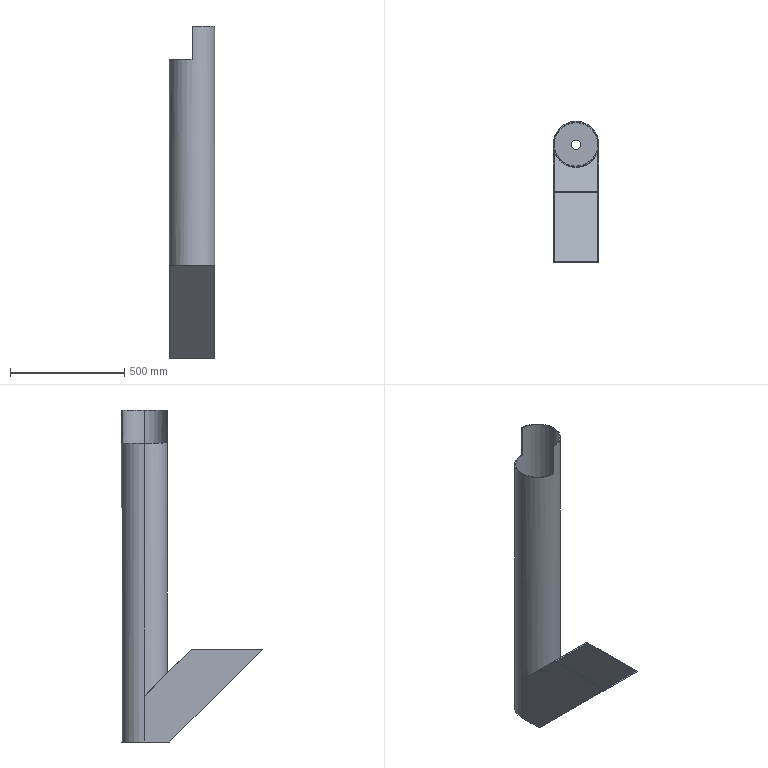Part | SolidWorks | features ICE 5, Shell 2, Extrusion 1 | 2 solids | 26 faces | box 200 x 616.127 x 1450 mm | volume 4635589 mm3 | plane 17 | cylinder 9 | commonest cylinder face diameters 192 x5 40 x2 200 x2
STEP:
#1=CARTESIAN_POINT('',(100.,0.,1450.));
#2=VERTEX_POINT('',#1);
#3=CARTESIAN_POINT('',(0.,100.,1450.));
#4=VERTEX_POINT('',#3);
#5=CARTESIAN_POINT('',(0.,0.,1450.));
#6=DIRECTION('',(0.,0.,1.));
#7=DIRECTION('',(1.,0.,0.));
#8=AXIS2_PLACEMENT_3D('',#5,#6,#7);
#9=CIRCLE('',#8,100.);
#10=EDGE_CURVE('',#2,#4,#9,.T.);
#11=ORIENTED_EDGE('',*,*,#10,.F.);
#12=CARTESIAN_POINT('',(100.,0.,200.));
#13=VERTEX_POINT('',#12);
#14=CARTESIAN_POINT('',(100.,0.,1450.));
#15=DIRECTION('',(0.,0.,-1.));
#16=VECTOR('',#15,1000.);
#17=LINE('',#14,#16);
#18=EDGE_CURVE('',#2,#13,#17,.T.);
#19=ORIENTED_EDGE('',*,*,#18,.T.);
#20=CARTESIAN_POINT('',(100.,0.,0.));
#21=VERTEX_POINT('',#20);
#22=CARTESIAN_POINT('',(100.,0.,0.));
#23=DIRECTION('',(0.,0.,1.));
#24=VECTOR('',#23,1000.);
#25=LINE('',#22,#24);
#26=EDGE_CURVE('',#21,#13,#25,.T.);
#27=ORIENTED_EDGE('',*,*,#26,.F.);
#28=CARTESIAN_POINT('',(-100.,0.,0.));
#29=VERTEX_POINT('',#28);
#30=CARTESIAN_POINT('',(0.,0.,0.));
#31=DIRECTION('',(0.,0.,1.));
#32=DIRECTION('',(1.,0.,0.));
#33=AXIS2_PLACEMENT_3D('',#30,#31,#32);
#34=CIRCLE('',#33,100.);
#35=EDGE_CURVE('',#21,#29,#34,.T.);
#36=ORIENTED_EDGE('',*,*,#35,.T.);
#37=CARTESIAN_POINT('',(-100.,0.,200.));
#38=VERTEX_POINT('',#37);
#39=CARTESIAN_POINT('',(-100.,0.,0.));
#40=DIRECTION('',(0.,0.,1.));
#41=VECTOR('',#40,1000.);
#42=LINE('',#39,#41);
#43=EDGE_CURVE('',#29,#38,#42,.T.);
#44=ORIENTED_EDGE('',*,*,#43,.T.);
#45=CARTESIAN_POINT('',(-100.,0.,1304.));
#46=VERTEX_POINT('',#45);
#47=CARTESIAN_POINT('',(-100.,0.,1450.));
#48=DIRECTION('',(0.,0.,-1.));
#49=VECTOR('',#48,1000.);
#50=LINE('',#47,#49);
#51=EDGE_CURVE('',#46,#38,#50,.T.);
#52=ORIENTED_EDGE('',*,*,#51,.F.);
#53=CARTESIAN_POINT('',(0.,100.,1304.));
#54=VERTEX_POINT('',#53);
#55=CARTESIAN_POINT('',(0.,0.,1304.));
#56=DIRECTION('',(0.,0.,1.));
#57=DIRECTION('',(1.,0.,0.));
#58=AXIS2_PLACEMENT_3D('',#55,#56,#57);
#59=CIRCLE('',#58,100.);
#60=EDGE_CURVE('',#54,#46,#59,.T.);
#61=ORIENTED_EDGE('',*,*,#60,.F.);
#62=CARTESIAN_POINT('',(0.,100.,1304.));
#63=DIRECTION('',(0.,0.,1.));
#64=VECTOR('',#63,1000.);
#65=LINE('',#62,#64);
#66=EDGE_CURVE('',#54,#4,#65,.T.);
#67=ORIENTED_EDGE('',*,*,#66,.T.);
#68=EDGE_LOOP('',(#11,#19,#27,#36,#44,#52,#61,#67));
#69=FACE_OUTER_BOUND('',#68,.T.);
#70=CARTESIAN_POINT('',(0.,0.,1450.));
#71=DIRECTION('',(0.,0.,-1.));
#72=DIRECTION('',(-1.,0.,0.));
#73=AXIS2_PLACEMENT_3D('',#70,#71,#72);
#74=CYLINDRICAL_SURFACE('',#73,100.);
#75=ADVANCED_FACE('',(#69),#74,.T.);
#76=CARTESIAN_POINT('',(0.,-96.,1450.));
#77=VERTEX_POINT('',#76);
#78=CARTESIAN_POINT('',(96.,0.,1450.));
#79=VERTEX_POINT('',#78);
#80=CARTESIAN_POINT('',(0.,0.,1450.));
#81=DIRECTION('',(0.,0.,1.));
#82=DIRECTION('',(1.,0.,0.));
#83=AXIS2_PLACEMENT_3D('',#80,#81,#82);
#84=CIRCLE('',#83,96.);
#85=EDGE_CURVE('',#77,#79,#84,.T.);
#86=ORIENTED_EDGE('',*,*,#85,.T.);
#87=CARTESIAN_POINT('',(96.,0.,194.343));
#88=VERTEX_POINT('',#87);
#89=CARTESIAN_POINT('',(96.,0.,1450.));
#90=DIRECTION('',(0.,0.,-1.));
#91=VECTOR('',#90,1000.);
#92=LINE('',#89,#91);
#93=EDGE_CURVE('',#79,#88,#92,.T.);
#94=ORIENTED_EDGE('',*,*,#93,.T.);
#95=CARTESIAN_POINT('',(-96.,0.,194.343));
#96=VERTEX_POINT('',#95);
#97=CARTESIAN_POINT('',(-96.,0.,194.343));
#98=CARTESIAN_POINT('',(-96.,-192.,386.343));
#99=CARTESIAN_POINT('',(96.,-192.,386.343));
#100=CARTESIAN_POINT('',(96.,0.,194.343));
#101=(BOUNDED_CURVE()B_SPLINE_CURVE(3,(#97,#98,#99,#100),.UNSPECIFIED.,.F.,.T.)B_SPLINE_CURVE_WITH_KNOTS((4,4),(1.571,4.712),.UNSPECIFIED.)CURVE()GEOMETRIC_REPRESENTATION_ITEM()RATIONAL_B_SPLINE_CURVE((1.,0.3333,0.3333,1.))REPRESENTATION_ITEM(''));
#102=EDGE_CURVE('',#96,#88,#101,.T.);
#103=ORIENTED_EDGE('',*,*,#102,.F.);
#104=CARTESIAN_POINT('',(-96.,0.,1304.));
#105=VERTEX_POINT('',#104);
#106=CARTESIAN_POINT('',(-96.,0.,1450.));
#107=DIRECTION('',(0.,0.,-1.));
#108=VECTOR('',#107,1000.);
#109=LINE('',#106,#108);
#110=EDGE_CURVE('',#105,#96,#109,.T.);
#111=ORIENTED_EDGE('',*,*,#110,.F.);
#112=CARTESIAN_POINT('',(0.,-96.,1304.));
#113=VERTEX_POINT('',#112);
#114=CARTESIAN_POINT('',(0.,0.,1304.));
#115=DIRECTION('',(0.,0.,1.));
#116=DIRECTION('',(1.,0.,0.));
#117=AXIS2_PLACEMENT_3D('',#114,#115,#116);
#118=CIRCLE('',#117,96.);
#119=EDGE_CURVE('',#105,#113,#118,.T.);
#120=ORIENTED_EDGE('',*,*,#119,.T.);
#121=CARTESIAN_POINT('',(0.,-96.,1450.));
#122=DIRECTION('',(0.,0.,-1.));
#123=VECTOR('',#122,1000.);
#124=LINE('',#121,#123);
#125=EDGE_CURVE('',#77,#113,#124,.T.);
#126=ORIENTED_EDGE('',*,*,#125,.F.);
#127=EDGE_LOOP('',(#86,#94,#103,#111,#120,#126));
#128=FACE_OUTER_BOUND('',#127,.T.);
#129=CARTESIAN_POINT('',(0.,0.,1450.));
#130=DIRECTION('',(0.,0.,-1.));
#131=DIRECTION('',(-1.,0.,0.));
#132=AXIS2_PLACEMENT_3D('',#129,#130,#131);
#133=CYLINDRICAL_SURFACE('',#132,96.);
#134=ADVANCED_FACE('',(#128),#133,.F.);
#135=CARTESIAN_POINT('',(-96.,0.,4.));
#136=VERTEX_POINT('',#135);
#137=CARTESIAN_POINT('',(96.,0.,4.));
#138=VERTEX_POINT('',#137);
#139=CARTESIAN_POINT('',(0.,0.,4.));
#140=DIRECTION('',(0.,0.,1.));
#141=DIRECTION('',(1.,0.,0.));
#142=AXIS2_PLACEMENT_3D('',#139,#140,#141);
#143=CIRCLE('',#142,96.);
#144=EDGE_CURVE('',#136,#138,#143,.T.);
#145=ORIENTED_EDGE('',*,*,#144,.T.);
#146=CARTESIAN_POINT('',(96.,0.,0.));
#147=VERTEX_POINT('',#146);
#148=CARTESIAN_POINT('',(96.,0.,1450.));
#149=DIRECTION('',(0.,0.,-1.));
#150=VECTOR('',#149,1000.);
#151=LINE('',#148,#150);
#152=EDGE_CURVE('',#138,#147,#151,.T.);
#153=ORIENTED_EDGE('',*,*,#152,.T.);
#154=CARTESIAN_POINT('',(-96.,0.,0.));
#155=VERTEX_POINT('',#154);
#156=CARTESIAN_POINT('',(0.,0.,0.));
#157=DIRECTION('',(0.,0.,1.));
#158=DIRECTION('',(1.,0.,0.));
#159=AXIS2_PLACEMENT_3D('',#156,#157,#158);
#160=CIRCLE('',#159,96.);
#161=EDGE_CURVE('',#155,#147,#160,.T.);
#162=ORIENTED_EDGE('',*,*,#161,.F.);
#163=CARTESIAN_POINT('',(-96.,0.,1450.));
#164=DIRECTION('',(0.,0.,-1.));
#165=VECTOR('',#164,1000.);
#166=LINE('',#163,#165);
#167=EDGE_CURVE('',#136,#155,#166,.T.);
#168=ORIENTED_EDGE('',*,*,#167,.F.);
#169=EDGE_LOOP('',(#145,#153,#162,#168));
#170=FACE_OUTER_BOUND('',#169,.T.);
#171=CARTESIAN_POINT('',(0.,0.,1450.));
#172=DIRECTION('',(0.,0.,-1.));
#173=DIRECTION('',(-1.,0.,0.));
#174=AXIS2_PLACEMENT_3D('',#171,#172,#173);
#175=CYLINDRICAL_SURFACE('',#174,96.);
#176=ADVANCED_FACE('',(#170),#175,.F.);
#177=ORIENTED_EDGE('',*,*,#93,.F.);
#178=CARTESIAN_POINT('',(0.,96.,1450.));
#179=VERTEX_POINT('',#178);
#180=CARTESIAN_POINT('',(0.,0.,1450.));
#181=DIRECTION('',(0.,0.,1.));
#182=DIRECTION('',(1.,0.,0.));
#183=AXIS2_PLACEMENT_3D('',#180,#181,#182);
#184=CIRCLE('',#183,96.);
#185=EDGE_CURVE('',#79,#179,#184,.T.);
#186=ORIENTED_EDGE('',*,*,#185,.T.);
#187=CARTESIAN_POINT('',(0.,96.,1304.));
#188=VERTEX_POINT('',#187);
#189=CARTESIAN_POINT('',(0.,96.,1450.));
#190=DIRECTION('',(0.,0.,1.));
#191=VECTOR('',#190,1000.);
#192=LINE('',#189,#191);
#193=EDGE_CURVE('',#188,#179,#192,.T.);
#194=ORIENTED_EDGE('',*,*,#193,.F.);
#195=CARTESIAN_POINT('',(0.,0.,1304.));
#196=DIRECTION('',(0.,0.,1.));
#197=DIRECTION('',(1.,0.,0.));
#198=AXIS2_PLACEMENT_3D('',#195,#196,#197);
#199=CIRCLE('',#198,96.);
#200=EDGE_CURVE('',#188,#105,#199,.T.);
#201=ORIENTED_EDGE('',*,*,#200,.T.);
#202=ORIENTED_EDGE('',*,*,#110,.T.);
#203=CARTESIAN_POINT('',(-96.,0.,1450.));
#204=DIRECTION('',(0.,0.,1.));
#205=VECTOR('',#204,1000.);
#206=LINE('',#203,#205);
#207=EDGE_CURVE('',#136,#96,#206,.T.);
#208=ORIENTED_EDGE('',*,*,#207,.F.);
#209=ORIENTED_EDGE('',*,*,#167,.T.);
#210=CARTESIAN_POINT('',(0.,0.,0.));
#211=DIRECTION('',(0.,0.,1.));
#212=DIRECTION('',(1.,0.,0.));
#213=AXIS2_PLACEMENT_3D('',#210,#211,#212);
#214=CIRCLE('',#213,96.);
#215=EDGE_CURVE('',#147,#155,#214,.T.);
#216=ORIENTED_EDGE('',*,*,#215,.F.);
#217=ORIENTED_EDGE('',*,*,#152,.F.);
#218=CARTESIAN_POINT('',(96.,0.,0.));
#219=DIRECTION('',(0.,0.,1.));
#220=VECTOR('',#219,1000.);
#221=LINE('',#218,#220);
#222=EDGE_CURVE('',#138,#88,#221,.T.);
#223=ORIENTED_EDGE('',*,*,#222,.T.);
#224=EDGE_LOOP('',(#177,#186,#194,#201,#202,#208,#209,#216,#217,#223));
#225=FACE_OUTER_BOUND('',#224,.T.);
#226=CARTESIAN_POINT('',(0.,0.,1450.));
#227=DIRECTION('',(0.,0.,-1.));
#228=DIRECTION('',(-1.,0.,0.));
#229=AXIS2_PLACEMENT_3D('',#226,#227,#228);
#230=CYLINDRICAL_SURFACE('',#229,96.);
#231=ADVANCED_FACE('',(#225),#230,.F.);
#232=CARTESIAN_POINT('',(-100.,-205.,405.));
#233=VERTEX_POINT('',#232);
#234=CARTESIAN_POINT('',(-100.,-516.127,405.));
#235=VERTEX_POINT('',#234);
#236=CARTESIAN_POINT('',(-100.,-205.,405.));
#237=DIRECTION('',(0.,-1.,0.));
#238=VECTOR('',#237,1000.);
#239=LINE('',#236,#238);
#240=EDGE_CURVE('',#233,#235,#239,.T.);
#241=ORIENTED_EDGE('',*,*,#240,.T.);
#242=CARTESIAN_POINT('',(100.,-516.127,405.));
#243=VERTEX_POINT('',#242);
#244=CARTESIAN_POINT('',(100.,-516.127,405.));
#245=DIRECTION('',(-1.,0.,0.));
#246=VECTOR('',#245,1000.);
#247=LINE('',#244,#246);
#248=EDGE_CURVE('',#243,#235,#247,.T.);
#249=ORIENTED_EDGE('',*,*,#248,.F.);
#250=CARTESIAN_POINT('',(100.,-205.,405.));
#251=VERTEX_POINT('',#250);
#252=CARTESIAN_POINT('',(100.,-205.,405.));
#253=DIRECTION('',(0.,-1.,0.));
#254=VECTOR('',#253,1000.);
#255=LINE('',#252,#254);
#256=EDGE_CURVE('',#251,#243,#255,.T.);
#257=ORIENTED_EDGE('',*,*,#256,.F.);
#258=CARTESIAN_POINT('',(100.,-205.,405.));
#259=DIRECTION('',(-1.,0.,0.));
#260=VECTOR('',#259,1000.);
#261=LINE('',#258,#260);
#262=EDGE_CURVE('',#251,#233,#261,.T.);
#263=ORIENTED_EDGE('',*,*,#262,.T.);
#264=EDGE_LOOP('',(#241,#249,#257,#263));
#265=FACE_OUTER_BOUND('',#264,.T.);
#266=CARTESIAN_POINT('',(-96.,-210.657,405.));
#267=VERTEX_POINT('',#266);
#268=CARTESIAN_POINT('',(-96.,-510.47,405.));
#269=VERTEX_POINT('',#268);
#270=CARTESIAN_POINT('',(-96.,0.,405.));
#271=DIRECTION('',(0.,-1.,0.));
#272=VECTOR('',#271,1000.);
#273=LINE('',#270,#272);
#274=EDGE_CURVE('',#267,#269,#273,.T.);
#275=ORIENTED_EDGE('',*,*,#274,.F.);
#276=CARTESIAN_POINT('',(96.,-210.657,405.));
#277=VERTEX_POINT('',#276);
#278=CARTESIAN_POINT('',(100.,-210.657,405.));
#279=DIRECTION('',(-1.,0.,0.));
#280=VECTOR('',#279,1000.);
#281=LINE('',#278,#280);
#282=EDGE_CURVE('',#277,#267,#281,.T.);
#283=ORIENTED_EDGE('',*,*,#282,.F.);
#284=CARTESIAN_POINT('',(96.,-510.47,405.));
#285=VERTEX_POINT('',#284);
#286=CARTESIAN_POINT('',(96.,0.,405.));
#287=DIRECTION('',(0.,-1.,0.));
#288=VECTOR('',#287,1000.);
#289=LINE('',#286,#288);
#290=EDGE_CURVE('',#277,#285,#289,.T.);
#291=ORIENTED_EDGE('',*,*,#290,.T.);
#292=CARTESIAN_POINT('',(100.,-510.47,405.));
#293=DIRECTION('',(-1.,0.,0.));
#294=VECTOR('',#293,1000.);
#295=LINE('',#292,#294);
#296=EDGE_CURVE('',#285,#269,#295,.T.);
#297=ORIENTED_EDGE('',*,*,#296,.T.);
#298=EDGE_LOOP('',(#275,#283,#291,#297));
#299=FACE_BOUND('',#298,.T.);
#300=CARTESIAN_POINT('',(100.,-205.,405.));
#301=DIRECTION('',(0.,0.,-1.));
#302=DIRECTION('',(-1.,0.,0.));
#303=AXIS2_PLACEMENT_3D('',#300,#301,#302);
#304=PLANE('',#303);
#305=ADVANCED_FACE('',(#265,#299),#304,.F.);
#306=ORIENTED_EDGE('',*,*,#18,.F.);
#307=CARTESIAN_POINT('',(0.,-100.,1450.));
#308=VERTEX_POINT('',#307);
#309=CARTESIAN_POINT('',(0.,0.,1450.));
#310=DIRECTION('',(0.,0.,1.));
#311=DIRECTION('',(1.,0.,0.));
#312=AXIS2_PLACEMENT_3D('',#309,#310,#311);
#313=CIRCLE('',#312,100.);
#314=EDGE_CURVE('',#308,#2,#313,.T.);
#315=ORIENTED_EDGE('',*,*,#314,.F.);
#316=CARTESIAN_POINT('',(0.,-100.,1304.));
#317=VERTEX_POINT('',#316);
#318=CARTESIAN_POINT('',(0.,-100.,1304.));
#319=DIRECTION('',(0.,0.,1.));
#320=VECTOR('',#319,1000.);
#321=LINE('',#318,#320);
#322=EDGE_CURVE('',#317,#308,#321,.T.);
#323=ORIENTED_EDGE('',*,*,#322,.F.);
#324=CARTESIAN_POINT('',(0.,0.,1304.));
#325=DIRECTION('',(0.,0.,1.));
#326=DIRECTION('',(1.,0.,0.));
#327=AXIS2_PLACEMENT_3D('',#324,#325,#326);
#328=CIRCLE('',#327,100.);
#329=EDGE_CURVE('',#46,#317,#328,.T.);
#330=ORIENTED_EDGE('',*,*,#329,.F.);
#331=ORIENTED_EDGE('',*,*,#51,.T.);
#332=CARTESIAN_POINT('',(-100.,0.,200.));
#333=CARTESIAN_POINT('',(-100.,-200.,400.));
#334=CARTESIAN_POINT('',(100.,-200.,400.));
#335=CARTESIAN_POINT('',(100.,0.,200.));
#336=(BOUNDED_CURVE()B_SPLINE_CURVE(3,(#332,#333,#334,#335),.UNSPECIFIED.,.F.,.T.)B_SPLINE_CURVE_WITH_KNOTS((4,4),(1.571,4.712),.UNSPECIFIED.)CURVE()GEOMETRIC_REPRESENTATION_ITEM()RATIONAL_B_SPLINE_CURVE((1.,0.3333,0.3333,1.))REPRESENTATION_ITEM(''));
#337=EDGE_CURVE('',#38,#13,#336,.T.);
#338=ORIENTED_EDGE('',*,*,#337,.T.);
#339=EDGE_LOOP('',(#306,#315,#323,#330,#331,#338));
#340=FACE_OUTER_BOUND('',#339,.T.);
#341=CARTESIAN_POINT('',(0.,0.,1450.));
#342=DIRECTION('',(0.,0.,-1.));
#343=DIRECTION('',(-1.,0.,0.));
#344=AXIS2_PLACEMENT_3D('',#341,#342,#343);
#345=CYLINDRICAL_SURFACE('',#344,100.);
#346=ADVANCED_FACE('',(#340),#345,.T.);
#347=CARTESIAN_POINT('',(0.,100.,1450.));
#348=DIRECTION('',(0.,1.,0.));
#349=VECTOR('',#348,1000.);
#350=LINE('',#347,#349);
#351=EDGE_CURVE('',#308,#77,#350,.T.);
#352=ORIENTED_EDGE('',*,*,#351,.F.);
#353=ORIENTED_EDGE('',*,*,#314,.T.);
#354=ORIENTED_EDGE('',*,*,#10,.T.);
#355=CARTESIAN_POINT('',(0.,100.,1450.));
#356=DIRECTION('',(0.,1.,0.));
#357=VECTOR('',#356,1000.);
#358=LINE('',#355,#357);
#359=EDGE_CURVE('',#179,#4,#358,.T.);
#360=ORIENTED_EDGE('',*,*,#359,.F.);
#361=ORIENTED_EDGE('',*,*,#185,.F.);
#362=ORIENTED_EDGE('',*,*,#85,.F.);
#363=EDGE_LOOP('',(#352,#353,#354,#360,#361,#362));
#364=FACE_OUTER_BOUND('',#363,.T.);
#365=CARTESIAN_POINT('',(0.,0.,1450.));
#366=DIRECTION('',(0.,0.,1.));
#367=DIRECTION('',(1.,0.,0.));
#368=AXIS2_PLACEMENT_3D('',#365,#366,#367);
#369=PLANE('',#368);
#370=ADVANCED_FACE('',(#364),#369,.T.);
#371=ORIENTED_EDGE('',*,*,#161,.T.);
#372=ORIENTED_EDGE('',*,*,#215,.T.);
#373=EDGE_LOOP('',(#371,#372));
#374=FACE_BOUND('',#373,.T.);
#375=ORIENTED_EDGE('',*,*,#35,.F.);
#376=CARTESIAN_POINT('',(100.,-111.127,0.));
#377=VERTEX_POINT('',#376);
#378=CARTESIAN_POINT('',(100.,0.,0.));
#379=DIRECTION('',(0.,-1.,0.));
#380=VECTOR('',#379,1000.);
#381=LINE('',#378,#380);
#382=EDGE_CURVE('',#21,#377,#381,.T.);
#383=ORIENTED_EDGE('',*,*,#382,.T.);
#384=CARTESIAN_POINT('',(-100.,-111.127,0.));
#385=VERTEX_POINT('',#384);
#386=CARTESIAN_POINT('',(100.,-111.127,0.));
#387=DIRECTION('',(-1.,0.,0.));
#388=VECTOR('',#387,1000.);
#389=LINE('',#386,#388);
#390=EDGE_CURVE('',#377,#385,#389,.T.);
#391=ORIENTED_EDGE('',*,*,#390,.T.);
#392=CARTESIAN_POINT('',(-100.,0.,0.));
#393=DIRECTION('',(0.,-1.,0.));
#394=VECTOR('',#393,1000.);
#395=LINE('',#392,#394);
#396=EDGE_CURVE('',#29,#385,#395,.T.);
#397=ORIENTED_EDGE('',*,*,#396,.F.);
#398=EDGE_LOOP('',(#375,#383,#391,#397));
#399=FACE_OUTER_BOUND('',#398,.T.);
#400=CARTESIAN_POINT('',(0.,0.,0.));
#401=DIRECTION('',(0.,0.,1.));
#402=DIRECTION('',(1.,0.,0.));
#403=AXIS2_PLACEMENT_3D('',#400,#401,#402);
#404=PLANE('',#403);
#405=ADVANCED_FACE('',(#374,#399),#404,.F.);
#406=ORIENTED_EDGE('',*,*,#125,.T.);
#407=CARTESIAN_POINT('',(0.,100.,1304.));
#408=DIRECTION('',(0.,1.,0.));
#409=VECTOR('',#408,1000.);
#410=LINE('',#407,#409);
#411=EDGE_CURVE('',#317,#113,#410,.T.);
#412=ORIENTED_EDGE('',*,*,#411,.F.);
#413=ORIENTED_EDGE('',*,*,#322,.T.);
#414=ORIENTED_EDGE('',*,*,#351,.T.);
#415=EDGE_LOOP('',(#406,#412,#413,#414));
#416=FACE_OUTER_BOUND('',#415,.T.);
#417=CARTESIAN_POINT('',(0.,100.,1304.));
#418=DIRECTION('',(1.,0.,0.));
#419=DIRECTION('',(0.,0.,-1.));
#420=AXIS2_PLACEMENT_3D('',#417,#418,#419);
#421=PLANE('',#420);
#422=ADVANCED_FACE('',(#416),#421,.F.);
#423=ORIENTED_EDGE('',*,*,#60,.T.);
#424=ORIENTED_EDGE('',*,*,#329,.T.);
#425=ORIENTED_EDGE('',*,*,#411,.T.);
#426=ORIENTED_EDGE('',*,*,#119,.F.);
#427=ORIENTED_EDGE('',*,*,#200,.F.);
#428=CARTESIAN_POINT('',(0.,100.,1304.));
#429=DIRECTION('',(0.,1.,0.));
#430=VECTOR('',#429,1000.);
#431=LINE('',#428,#430);
#432=EDGE_CURVE('',#188,#54,#431,.T.);
#433=ORIENTED_EDGE('',*,*,#432,.T.);
#434=EDGE_LOOP('',(#423,#424,#425,#426,#427,#433));
#435=FACE_OUTER_BOUND('',#434,.T.);
#436=CARTESIAN_POINT('',(0.,0.,1304.));
#437=DIRECTION('',(0.,0.,1.));
#438=DIRECTION('',(1.,0.,0.));
#439=AXIS2_PLACEMENT_3D('',#436,#437,#438);
#440=PLANE('',#439);
#441=ADVANCED_FACE('',(#435),#440,.T.);
#442=ORIENTED_EDGE('',*,*,#193,.T.);
#443=ORIENTED_EDGE('',*,*,#359,.T.);
#444=ORIENTED_EDGE('',*,*,#66,.F.);
#445=ORIENTED_EDGE('',*,*,#432,.F.);
#446=EDGE_LOOP('',(#442,#443,#444,#445));
#447=FACE_OUTER_BOUND('',#446,.T.);
#448=CARTESIAN_POINT('',(0.,100.,1304.));
#449=DIRECTION('',(1.,0.,0.));
#450=DIRECTION('',(0.,0.,-1.));
#451=AXIS2_PLACEMENT_3D('',#448,#449,#450);
#452=PLANE('',#451);
#453=ADVANCED_FACE('',(#447),#452,.F.);
#454=ORIENTED_EDGE('',*,*,#396,.T.);
#455=CARTESIAN_POINT('',(-100.,-111.127,0.));
#456=DIRECTION('',(0.,-0.7071,0.7071));
#457=VECTOR('',#456,1000.);
#458=LINE('',#455,#457);
#459=EDGE_CURVE('',#385,#235,#458,.T.);
#460=ORIENTED_EDGE('',*,*,#459,.T.);
#461=ORIENTED_EDGE('',*,*,#240,.F.);
#462=CARTESIAN_POINT('',(-100.,0.,200.));
#463=DIRECTION('',(0.,-0.7071,0.7071));
#464=VECTOR('',#463,1000.);
#465=LINE('',#462,#464);
#466=EDGE_CURVE('',#38,#233,#465,.T.);
#467=ORIENTED_EDGE('',*,*,#466,.F.);
#468=ORIENTED_EDGE('',*,*,#43,.F.);
#469=EDGE_LOOP('',(#454,#460,#461,#467,#468));
#470=FACE_OUTER_BOUND('',#469,.T.);
#471=CARTESIAN_POINT('',(-100.,0.,0.));
#472=DIRECTION('',(-1.,0.,0.));
#473=DIRECTION('',(0.,0.,1.));
#474=AXIS2_PLACEMENT_3D('',#471,#472,#473);
#475=PLANE('',#474);
#476=ADVANCED_FACE('',(#470),#475,.T.);
#477=ORIENTED_EDGE('',*,*,#382,.F.);
#478=ORIENTED_EDGE('',*,*,#26,.T.);
#479=CARTESIAN_POINT('',(100.,-100.,300.));
#480=DIRECTION('',(0.,-0.7071,0.7071));
#481=VECTOR('',#480,1000.);
#482=LINE('',#479,#481);
#483=EDGE_CURVE('',#13,#251,#482,.T.);
#484=ORIENTED_EDGE('',*,*,#483,.T.);
#485=ORIENTED_EDGE('',*,*,#256,.T.);
#486=CARTESIAN_POINT('',(100.,-111.127,0.));
#487=DIRECTION('',(0.,-0.7071,0.7071));
#488=VECTOR('',#487,1000.);
#489=LINE('',#486,#488);
#490=EDGE_CURVE('',#377,#243,#489,.T.);
#491=ORIENTED_EDGE('',*,*,#490,.F.);
#492=EDGE_LOOP('',(#477,#478,#484,#485,#491));
#493=FACE_OUTER_BOUND('',#492,.T.);
#494=CARTESIAN_POINT('',(100.,0.,0.));
#495=DIRECTION('',(-1.,0.,0.));
#496=DIRECTION('',(0.,0.,1.));
#497=AXIS2_PLACEMENT_3D('',#494,#495,#496);
#498=PLANE('',#497);
#499=ADVANCED_FACE('',(#493),#498,.F.);
#500=ORIENTED_EDGE('',*,*,#459,.F.);
#501=ORIENTED_EDGE('',*,*,#390,.F.);
#502=ORIENTED_EDGE('',*,*,#490,.T.);
#503=ORIENTED_EDGE('',*,*,#248,.T.);
#504=EDGE_LOOP('',(#500,#501,#502,#503));
#505=FACE_OUTER_BOUND('',#504,.T.);
#506=CARTESIAN_POINT('',(100.,-111.127,0.));
#507=DIRECTION('',(0.,-0.7071,-0.7071));
#508=DIRECTION('',(0.,0.7071,-0.7071));
#509=AXIS2_PLACEMENT_3D('',#506,#507,#508);
#510=PLANE('',#509);
#511=ADVANCED_FACE('',(#505),#510,.T.);
#512=ORIENTED_EDGE('',*,*,#483,.F.);
#513=ORIENTED_EDGE('',*,*,#337,.F.);
#514=ORIENTED_EDGE('',*,*,#466,.T.);
#515=ORIENTED_EDGE('',*,*,#262,.F.);
#516=EDGE_LOOP('',(#512,#513,#514,#515));
#517=FACE_OUTER_BOUND('',#516,.T.);
#518=CARTESIAN_POINT('',(100.,0.,200.));
#519=DIRECTION('',(0.,-0.7071,-0.7071));
#520=DIRECTION('',(0.,0.7071,-0.7071));
#521=AXIS2_PLACEMENT_3D('',#518,#519,#520);
#522=PLANE('',#521);
#523=ADVANCED_FACE('',(#517),#522,.F.);
#524=ORIENTED_EDGE('',*,*,#144,.F.);
#525=CARTESIAN_POINT('',(-96.,-109.47,4.));
#526=VERTEX_POINT('',#525);
#527=CARTESIAN_POINT('',(-96.,0.,4.));
#528=DIRECTION('',(0.,-1.,0.));
#529=VECTOR('',#528,1000.);
#530=LINE('',#527,#529);
#531=EDGE_CURVE('',#136,#526,#530,.T.);
#532=ORIENTED_EDGE('',*,*,#531,.T.);
#533=CARTESIAN_POINT('',(96.,-109.47,4.));
#534=VERTEX_POINT('',#533);
#535=CARTESIAN_POINT('',(100.,-109.47,4.));
#536=DIRECTION('',(-1.,0.,0.));
#537=VECTOR('',#536,1000.);
#538=LINE('',#535,#537);
#539=EDGE_CURVE('',#534,#526,#538,.T.);
#540=ORIENTED_EDGE('',*,*,#539,.F.);
#541=CARTESIAN_POINT('',(96.,0.,4.));
#542=DIRECTION('',(0.,-1.,0.));
#543=VECTOR('',#542,1000.);
#544=LINE('',#541,#543);
#545=EDGE_CURVE('',#138,#534,#544,.T.);
#546=ORIENTED_EDGE('',*,*,#545,.F.);
#547=EDGE_LOOP('',(#524,#532,#540,#546));
#548=FACE_OUTER_BOUND('',#547,.T.);
#549=CARTESIAN_POINT('',(0.,0.,4.));
#550=DIRECTION('',(0.,0.,1.));
#551=DIRECTION('',(1.,0.,0.));
#552=AXIS2_PLACEMENT_3D('',#549,#550,#551);
#553=PLANE('',#552);
#554=ADVANCED_FACE('',(#548),#553,.T.);
#555=ORIENTED_EDGE('',*,*,#531,.F.);
#556=ORIENTED_EDGE('',*,*,#207,.T.);
#557=CARTESIAN_POINT('',(-96.,97.172,97.172));
#558=DIRECTION('',(0.,-0.7071,0.7071));
#559=VECTOR('',#558,1000.);
#560=LINE('',#557,#559);
#561=EDGE_CURVE('',#96,#267,#560,.T.);
#562=ORIENTED_EDGE('',*,*,#561,.T.);
#563=ORIENTED_EDGE('',*,*,#274,.T.);
#564=CARTESIAN_POINT('',(-96.,-52.735,-52.735));
#565=DIRECTION('',(0.,-0.7071,0.7071));
#566=VECTOR('',#565,1000.);
#567=LINE('',#564,#566);
#568=EDGE_CURVE('',#526,#269,#567,.T.);
#569=ORIENTED_EDGE('',*,*,#568,.F.);
#570=EDGE_LOOP('',(#555,#556,#562,#563,#569));
#571=FACE_OUTER_BOUND('',#570,.T.);
#572=CARTESIAN_POINT('',(-96.,0.,0.));
#573=DIRECTION('',(-1.,0.,0.));
#574=DIRECTION('',(0.,0.,1.));
#575=AXIS2_PLACEMENT_3D('',#572,#573,#574);
#576=PLANE('',#575);
#577=ADVANCED_FACE('',(#571),#576,.F.);
#578=ORIENTED_EDGE('',*,*,#545,.T.);
#579=CARTESIAN_POINT('',(96.,-52.735,-52.735));
#580=DIRECTION('',(0.,-0.7071,0.7071));
#581=VECTOR('',#580,1000.);
#582=LINE('',#579,#581);
#583=EDGE_CURVE('',#534,#285,#582,.T.);
#584=ORIENTED_EDGE('',*,*,#583,.T.);
#585=ORIENTED_EDGE('',*,*,#290,.F.);
#586=CARTESIAN_POINT('',(96.,97.172,97.172));
#587=DIRECTION('',(0.,-0.7071,0.7071));
#588=VECTOR('',#587,1000.);
#589=LINE('',#586,#588);
#590=EDGE_CURVE('',#88,#277,#589,.T.);
#591=ORIENTED_EDGE('',*,*,#590,.F.);
#592=ORIENTED_EDGE('',*,*,#222,.F.);
#593=EDGE_LOOP('',(#578,#584,#585,#591,#592));
#594=FACE_OUTER_BOUND('',#593,.T.);
#595=CARTESIAN_POINT('',(96.,0.,0.));
#596=DIRECTION('',(-1.,0.,0.));
#597=DIRECTION('',(0.,0.,1.));
#598=AXIS2_PLACEMENT_3D('',#595,#596,#597);
#599=PLANE('',#598);
#600=ADVANCED_FACE('',(#594),#599,.T.);
#601=ORIENTED_EDGE('',*,*,#568,.T.);
#602=ORIENTED_EDGE('',*,*,#296,.F.);
#603=ORIENTED_EDGE('',*,*,#583,.F.);
#604=ORIENTED_EDGE('',*,*,#539,.T.);
#605=EDGE_LOOP('',(#601,#602,#603,#604));
#606=FACE_OUTER_BOUND('',#605,.T.);
#607=CARTESIAN_POINT('',(100.,-108.299,2.828));
#608=DIRECTION('',(0.,-0.7071,-0.7071));
#609=DIRECTION('',(0.,0.7071,-0.7071));
#610=AXIS2_PLACEMENT_3D('',#607,#608,#609);
#611=PLANE('',#610);
#612=ADVANCED_FACE('',(#606),#611,.F.);
#613=ORIENTED_EDGE('',*,*,#590,.T.);
#614=ORIENTED_EDGE('',*,*,#282,.T.);
#615=ORIENTED_EDGE('',*,*,#561,.F.);
#616=ORIENTED_EDGE('',*,*,#102,.T.);
#617=EDGE_LOOP('',(#613,#614,#615,#616));
#618=FACE_OUTER_BOUND('',#617,.T.);
#619=CARTESIAN_POINT('',(100.,-2.828,197.172));
#620=DIRECTION('',(0.,-0.7071,-0.7071));
#621=DIRECTION('',(0.,0.7071,-0.7071));
#622=AXIS2_PLACEMENT_3D('',#619,#620,#621);
#623=PLANE('',#622);
#624=ADVANCED_FACE('',(#618),#623,.T.);
#625=CLOSED_SHELL('',(#75,#134,#176,#231,#305,#346,#370,#405,#422,#441,#453,#476,#499,#511,#523,#554,#577,#600,#612,#624));
#626=MANIFOLD_SOLID_BREP('',#625);
#627=CARTESIAN_POINT('',(20.,0.,4.));
#628=VERTEX_POINT('',#627);
#629=CARTESIAN_POINT('',(-20.,0.,4.));
#630=VERTEX_POINT('',#629);
#631=CARTESIAN_POINT('',(0.,0.,4.));
#632=DIRECTION('',(0.,0.,-1.));
#633=DIRECTION('',(-1.,0.,0.));
#634=AXIS2_PLACEMENT_3D('',#631,#632,#633);
#635=CIRCLE('',#634,20.);
#636=EDGE_CURVE('',#628,#630,#635,.T.);
#637=ORIENTED_EDGE('',*,*,#636,.F.);
#638=CARTESIAN_POINT('',(20.,0.,0.));
#639=VERTEX_POINT('',#638);
#640=CARTESIAN_POINT('',(20.,0.,4.));
#641=DIRECTION('',(0.,0.,-1.));
#642=VECTOR('',#641,1000.);
#643=LINE('',#640,#642);
#644=EDGE_CURVE('',#628,#639,#643,.T.);
#645=ORIENTED_EDGE('',*,*,#644,.T.);
#646=CARTESIAN_POINT('',(-20.,0.,0.));
#647=VERTEX_POINT('',#646);
#648=CARTESIAN_POINT('',(0.,0.,0.));
#649=DIRECTION('',(0.,0.,-1.));
#650=DIRECTION('',(-1.,0.,0.));
#651=AXIS2_PLACEMENT_3D('',#648,#649,#650);
#652=CIRCLE('',#651,20.);
#653=EDGE_CURVE('',#639,#647,#652,.T.);
#654=ORIENTED_EDGE('',*,*,#653,.T.);
#655=CARTESIAN_POINT('',(-20.,0.,4.));
#656=DIRECTION('',(0.,0.,-1.));
#657=VECTOR('',#656,1000.);
#658=LINE('',#655,#657);
#659=EDGE_CURVE('',#630,#647,#658,.T.);
#660=ORIENTED_EDGE('',*,*,#659,.F.);
#661=EDGE_LOOP('',(#637,#645,#654,#660));
#662=FACE_OUTER_BOUND('',#661,.T.);
#663=CARTESIAN_POINT('',(0.,0.,4.));
#664=DIRECTION('',(0.,0.,-1.));
#665=DIRECTION('',(-1.,0.,0.));
#666=AXIS2_PLACEMENT_3D('',#663,#664,#665);
#667=CYLINDRICAL_SURFACE('',#666,20.);
#668=ADVANCED_FACE('',(#662),#667,.F.);
#669=CARTESIAN_POINT('',(-96.,0.,4.));
#670=VERTEX_POINT('',#669);
#671=CARTESIAN_POINT('',(96.,0.,4.));
#672=VERTEX_POINT('',#671);
#673=CARTESIAN_POINT('',(0.,0.,4.));
#674=DIRECTION('',(0.,0.,-1.));
#675=DIRECTION('',(-1.,0.,0.));
#676=AXIS2_PLACEMENT_3D('',#673,#674,#675);
#677=CIRCLE('',#676,96.);
#678=EDGE_CURVE('',#670,#672,#677,.T.);
#679=ORIENTED_EDGE('',*,*,#678,.T.);
#680=CARTESIAN_POINT('',(96.,0.,0.));
#681=VERTEX_POINT('',#680);
#682=CARTESIAN_POINT('',(96.,0.,4.));
#683=DIRECTION('',(0.,0.,-1.));
#684=VECTOR('',#683,1000.);
#685=LINE('',#682,#684);
#686=EDGE_CURVE('',#672,#681,#685,.T.);
#687=ORIENTED_EDGE('',*,*,#686,.T.);
#688=CARTESIAN_POINT('',(-96.,0.,0.));
#689=VERTEX_POINT('',#688);
#690=CARTESIAN_POINT('',(0.,0.,0.));
#691=DIRECTION('',(0.,0.,-1.));
#692=DIRECTION('',(-1.,0.,0.));
#693=AXIS2_PLACEMENT_3D('',#690,#691,#692);
#694=CIRCLE('',#693,96.);
#695=EDGE_CURVE('',#689,#681,#694,.T.);
#696=ORIENTED_EDGE('',*,*,#695,.F.);
#697=CARTESIAN_POINT('',(-96.,0.,4.));
#698=DIRECTION('',(0.,0.,-1.));
#699=VECTOR('',#698,1000.);
#700=LINE('',#697,#699);
#701=EDGE_CURVE('',#670,#689,#700,.T.);
#702=ORIENTED_EDGE('',*,*,#701,.F.);
#703=EDGE_LOOP('',(#679,#687,#696,#702));
#704=FACE_OUTER_BOUND('',#703,.T.);
#705=CARTESIAN_POINT('',(0.,0.,4.));
#706=DIRECTION('',(0.,0.,-1.));
#707=DIRECTION('',(-1.,0.,0.));
#708=AXIS2_PLACEMENT_3D('',#705,#706,#707);
#709=CYLINDRICAL_SURFACE('',#708,96.);
#710=ADVANCED_FACE('',(#704),#709,.T.);
#711=ORIENTED_EDGE('',*,*,#686,.F.);
#712=CARTESIAN_POINT('',(0.,0.,4.));
#713=DIRECTION('',(0.,0.,-1.));
#714=DIRECTION('',(-1.,0.,0.));
#715=AXIS2_PLACEMENT_3D('',#712,#713,#714);
#716=CIRCLE('',#715,96.);
#717=EDGE_CURVE('',#672,#670,#716,.T.);
#718=ORIENTED_EDGE('',*,*,#717,.T.);
#719=ORIENTED_EDGE('',*,*,#701,.T.);
#720=CARTESIAN_POINT('',(0.,0.,0.));
#721=DIRECTION('',(0.,0.,-1.));
#722=DIRECTION('',(-1.,0.,0.));
#723=AXIS2_PLACEMENT_3D('',#720,#721,#722);
#724=CIRCLE('',#723,96.);
#725=EDGE_CURVE('',#681,#689,#724,.T.);
#726=ORIENTED_EDGE('',*,*,#725,.F.);
#727=EDGE_LOOP('',(#711,#718,#719,#726));
#728=FACE_OUTER_BOUND('',#727,.T.);
#729=CARTESIAN_POINT('',(0.,0.,4.));
#730=DIRECTION('',(0.,0.,-1.));
#731=DIRECTION('',(-1.,0.,0.));
#732=AXIS2_PLACEMENT_3D('',#729,#730,#731);
#733=CYLINDRICAL_SURFACE('',#732,96.);
#734=ADVANCED_FACE('',(#728),#733,.T.);
#735=CARTESIAN_POINT('',(0.,0.,4.));
#736=DIRECTION('',(0.,0.,-1.));
#737=DIRECTION('',(-1.,0.,0.));
#738=AXIS2_PLACEMENT_3D('',#735,#736,#737);
#739=CIRCLE('',#738,20.);
#740=EDGE_CURVE('',#630,#628,#739,.T.);
#741=ORIENTED_EDGE('',*,*,#740,.T.);
#742=ORIENTED_EDGE('',*,*,#636,.T.);
#743=EDGE_LOOP('',(#741,#742));
#744=FACE_BOUND('',#743,.T.);
#745=ORIENTED_EDGE('',*,*,#678,.F.);
#746=ORIENTED_EDGE('',*,*,#717,.F.);
#747=EDGE_LOOP('',(#745,#746));
#748=FACE_OUTER_BOUND('',#747,.T.);
#749=CARTESIAN_POINT('',(0.,0.,4.));
#750=DIRECTION('',(0.,0.,-1.));
#751=DIRECTION('',(-1.,0.,0.));
#752=AXIS2_PLACEMENT_3D('',#749,#750,#751);
#753=PLANE('',#752);
#754=ADVANCED_FACE('',(#744,#748),#753,.F.);
#755=CARTESIAN_POINT('',(0.,0.,0.));
#756=DIRECTION('',(0.,0.,-1.));
#757=DIRECTION('',(-1.,0.,0.));
#758=AXIS2_PLACEMENT_3D('',#755,#756,#757);
#759=CIRCLE('',#758,20.);
#760=EDGE_CURVE('',#647,#639,#759,.T.);
#761=ORIENTED_EDGE('',*,*,#760,.F.);
#762=ORIENTED_EDGE('',*,*,#653,.F.);
#763=EDGE_LOOP('',(#761,#762));
#764=FACE_BOUND('',#763,.T.);
#765=ORIENTED_EDGE('',*,*,#695,.T.);
#766=ORIENTED_EDGE('',*,*,#725,.T.);
#767=EDGE_LOOP('',(#765,#766));
#768=FACE_OUTER_BOUND('',#767,.T.);
#769=CARTESIAN_POINT('',(0.,0.,0.));
#770=DIRECTION('',(0.,0.,-1.));
#771=DIRECTION('',(-1.,0.,0.));
#772=AXIS2_PLACEMENT_3D('',#769,#770,#771);
#773=PLANE('',#772);
#774=ADVANCED_FACE('',(#764,#768),#773,.T.);
#775=ORIENTED_EDGE('',*,*,#644,.F.);
#776=ORIENTED_EDGE('',*,*,#740,.F.);
#777=ORIENTED_EDGE('',*,*,#659,.T.);
#778=ORIENTED_EDGE('',*,*,#760,.T.);
#779=EDGE_LOOP('',(#775,#776,#777,#778));
#780=FACE_OUTER_BOUND('',#779,.T.);
#781=CARTESIAN_POINT('',(0.,0.,4.));
#782=DIRECTION('',(0.,0.,-1.));
#783=DIRECTION('',(-1.,0.,0.));
#784=AXIS2_PLACEMENT_3D('',#781,#782,#783);
#785=CYLINDRICAL_SURFACE('',#784,20.);
#786=ADVANCED_FACE('',(#780),#785,.F.);
#787=CLOSED_SHELL('',(#668,#710,#734,#754,#774,#786));
#788=MANIFOLD_SOLID_BREP('',#787);
#789=CARTESIAN_POINT('',(0.,0.,0.));
#790=DIRECTION('',(0.,0.,1.));
#791=DIRECTION('',(1.,0.,0.));
#792=AXIS2_PLACEMENT_3D('',#789,#790,#791);
#793=(LENGTH_UNIT()NAMED_UNIT(*)SI_UNIT(.MILLI.,.METRE.));
#794=UNCERTAINTY_MEASURE_WITH_UNIT(LENGTH_MEASURE(0.00001),#793,'','');
#795=(NAMED_UNIT(*)PLANE_ANGLE_UNIT()SI_UNIT($,.RADIAN.));
#796=(NAMED_UNIT(*)SI_UNIT($,.STERADIAN.)SOLID_ANGLE_UNIT());
#797=(GEOMETRIC_REPRESENTATION_CONTEXT(3)GLOBAL_UNCERTAINTY_ASSIGNED_CONTEXT((#794))GLOBAL_UNIT_ASSIGNED_CONTEXT((#793,#795,#796))REPRESENTATION_CONTEXT('',''));
#798=ADVANCED_BREP_SHAPE_REPRESENTATION('',(#626,#788,#792),#797);